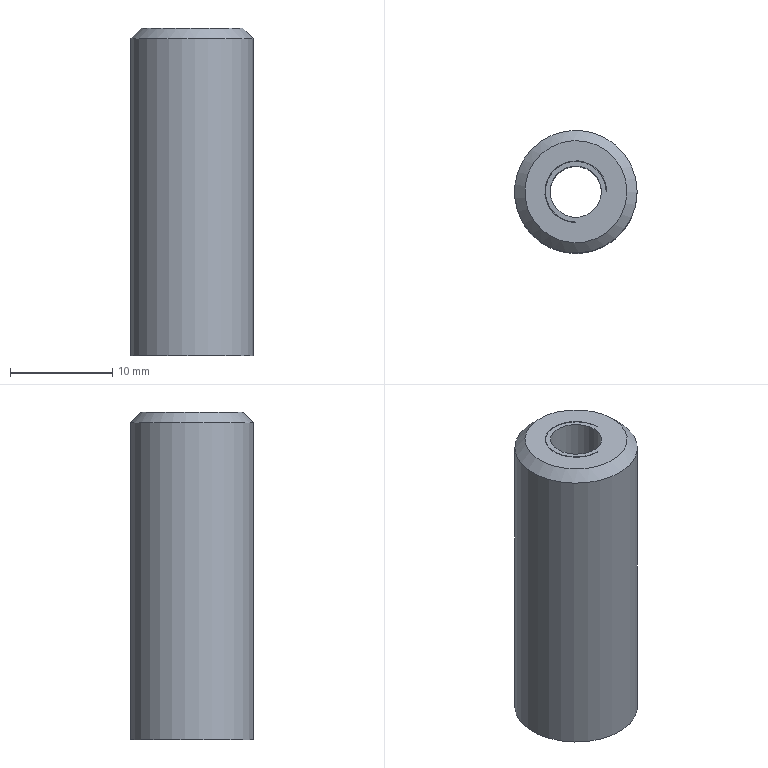Part | STEP file | Tube necking machine_id26_x_t | 1 solid | 9 faces | box 12 x 12 x 32 mm | volume 2950 mm3 | cylinder 4 | plane 4 | cone 1 | commonest cylinder face diameters 5 x1 5.95 x1 6.05 x1 12 x1
STEP:
#1=CARTESIAN_POINT('',(0.,0.,0.));
#2=DIRECTION('',(0.,0.,1.));
#3=DIRECTION('',(1.,0.,0.));
#4=AXIS2_PLACEMENT_3D('',#1,#2,#3);
#5=CARTESIAN_POINT('',(2.975,50.,73.));
#6=VERTEX_POINT('',#5);
#7=CARTESIAN_POINT('',(2.975,50.,105.));
#8=VERTEX_POINT('',#7);
#9=CARTESIAN_POINT('',(2.975,50.,92.));
#10=DIRECTION('',(0.,0.,1.));
#11=VECTOR('',#10,1.);
#12=LINE('',#9,#11);
#13=CARTESIAN_POINT('',(0.,50.,92.));
#14=DIRECTION('',(0.,0.,-1.));
#15=DIRECTION('',(1.,0.,0.));
#16=AXIS2_PLACEMENT_3D('',#13,#14,#15);
#17=CYLINDRICAL_SURFACE('',#16,2.975);
#18=CARTESIAN_POINT('',(6.283,0.));
#19=DIRECTION('',(0.,-1.));
#20=VECTOR('',#19,1.);
#21=LINE('',#18,#20);
#22=(GEOMETRIC_REPRESENTATION_CONTEXT(2)PARAMETRIC_REPRESENTATION_CONTEXT()REPRESENTATION_CONTEXT('',''));
#23=DEFINITIONAL_REPRESENTATION('',(#21),#22);
#24=PCURVE('',#17,#23);
#25=CARTESIAN_POINT('',(3.,50.,85.5));
#26=DIRECTION('',(0.,-1.,0.));
#27=DIRECTION('',(0.,0.,-1.));
#28=AXIS2_PLACEMENT_3D('',#25,#26,#27);
#29=PLANE('',#28);
#30=CARTESIAN_POINT('',(-6.5,-0.025));
#31=DIRECTION('',(-1.,0.));
#32=VECTOR('',#31,1.);
#33=LINE('',#30,#32);
#34=(GEOMETRIC_REPRESENTATION_CONTEXT(2)PARAMETRIC_REPRESENTATION_CONTEXT()REPRESENTATION_CONTEXT('',''));
#35=DEFINITIONAL_REPRESENTATION('',(#33),#34);
#36=PCURVE('',#29,#35);
#37=SURFACE_CURVE('',#12,(#24,#36),.PCURVE_S1.);
#38=EDGE_CURVE('',#6,#8,#37,.T.);
#39=ORIENTED_EDGE('',*,*,#38,.F.);
#40=CARTESIAN_POINT('',(0.,47.025,73.));
#41=VERTEX_POINT('',#40);
#42=CARTESIAN_POINT('',(0.,50.,73.));
#43=DIRECTION('',(0.,0.,1.));
#44=DIRECTION('',(1.,0.,0.));
#45=AXIS2_PLACEMENT_3D('',#42,#43,#44);
#46=CIRCLE('',#45,2.975);
#47=CARTESIAN_POINT('',(6.283,19.));
#48=DIRECTION('',(-1.,0.));
#49=VECTOR('',#48,1.);
#50=LINE('',#47,#49);
#51=(GEOMETRIC_REPRESENTATION_CONTEXT(2)PARAMETRIC_REPRESENTATION_CONTEXT()REPRESENTATION_CONTEXT('',''));
#52=DEFINITIONAL_REPRESENTATION('',(#50),#51);
#53=PCURVE('',#17,#52);
#54=CARTESIAN_POINT('',(0.,50.,73.));
#55=DIRECTION('',(0.,0.,1.));
#56=DIRECTION('',(1.,0.,0.));
#57=AXIS2_PLACEMENT_3D('',#54,#55,#56);
#58=PLANE('',#57);
#59=CARTESIAN_POINT('',(0.,0.));
#60=DIRECTION('',(1.,0.));
#61=AXIS2_PLACEMENT_2D('',#59,#60);
#62=CIRCLE('',#61,2.975);
#63=(GEOMETRIC_REPRESENTATION_CONTEXT(2)PARAMETRIC_REPRESENTATION_CONTEXT()REPRESENTATION_CONTEXT('',''));
#64=DEFINITIONAL_REPRESENTATION('',(#62),#63);
#65=PCURVE('',#58,#64);
#66=SURFACE_CURVE('',#46,(#53,#65),.PCURVE_S1.);
#67=EDGE_CURVE('',#6,#41,#66,.T.);
#68=ORIENTED_EDGE('',*,*,#67,.T.);
#69=CARTESIAN_POINT('',(0.,47.025,105.));
#70=VERTEX_POINT('',#69);
#71=CARTESIAN_POINT('',(0.,47.025,92.));
#72=DIRECTION('',(0.,0.,1.));
#73=VECTOR('',#72,1.);
#74=LINE('',#71,#73);
#75=CARTESIAN_POINT('',(1.571,0.));
#76=DIRECTION('',(0.,-1.));
#77=VECTOR('',#76,1.);
#78=LINE('',#75,#77);
#79=(GEOMETRIC_REPRESENTATION_CONTEXT(2)PARAMETRIC_REPRESENTATION_CONTEXT()REPRESENTATION_CONTEXT('',''));
#80=DEFINITIONAL_REPRESENTATION('',(#78),#79);
#81=PCURVE('',#17,#80);
#82=CARTESIAN_POINT('',(0.,47.,85.5));
#83=DIRECTION('',(-1.,0.,0.));
#84=DIRECTION('',(0.,0.,-1.));
#85=AXIS2_PLACEMENT_3D('',#82,#83,#84);
#86=PLANE('',#85);
#87=CARTESIAN_POINT('',(-6.5,-0.025));
#88=DIRECTION('',(-1.,0.));
#89=VECTOR('',#88,1.);
#90=LINE('',#87,#89);
#91=(GEOMETRIC_REPRESENTATION_CONTEXT(2)PARAMETRIC_REPRESENTATION_CONTEXT()REPRESENTATION_CONTEXT('',''));
#92=DEFINITIONAL_REPRESENTATION('',(#90),#91);
#93=PCURVE('',#86,#92);
#94=SURFACE_CURVE('',#74,(#81,#93),.PCURVE_S1.);
#95=EDGE_CURVE('',#41,#70,#94,.T.);
#96=ORIENTED_EDGE('',*,*,#95,.T.);
#97=CARTESIAN_POINT('',(0.,50.,105.));
#98=DIRECTION('',(0.,0.,1.));
#99=DIRECTION('',(1.,0.,0.));
#100=AXIS2_PLACEMENT_3D('',#97,#98,#99);
#101=CIRCLE('',#100,2.975);
#102=CARTESIAN_POINT('',(6.283,-13.));
#103=DIRECTION('',(-1.,0.));
#104=VECTOR('',#103,1.);
#105=LINE('',#102,#104);
#106=(GEOMETRIC_REPRESENTATION_CONTEXT(2)PARAMETRIC_REPRESENTATION_CONTEXT()REPRESENTATION_CONTEXT('',''));
#107=DEFINITIONAL_REPRESENTATION('',(#105),#106);
#108=PCURVE('',#17,#107);
#109=CARTESIAN_POINT('',(0.,50.,105.));
#110=DIRECTION('',(0.,0.,1.));
#111=DIRECTION('',(1.,0.,0.));
#112=AXIS2_PLACEMENT_3D('',#109,#110,#111);
#113=PLANE('',#112);
#114=CARTESIAN_POINT('',(0.,0.));
#115=DIRECTION('',(1.,0.));
#116=AXIS2_PLACEMENT_2D('',#114,#115);
#117=CIRCLE('',#116,2.975);
#118=(GEOMETRIC_REPRESENTATION_CONTEXT(2)PARAMETRIC_REPRESENTATION_CONTEXT()REPRESENTATION_CONTEXT('',''));
#119=DEFINITIONAL_REPRESENTATION('',(#117),#118);
#120=PCURVE('',#113,#119);
#121=SURFACE_CURVE('',#101,(#108,#120),.PCURVE_S1.);
#122=EDGE_CURVE('',#8,#70,#121,.T.);
#123=ORIENTED_EDGE('',*,*,#122,.F.);
#124=EDGE_LOOP('',(#39,#68,#96,#123));
#125=FACE_BOUND('',#124,.T.);
#126=ADVANCED_FACE('',(#125),#17,.T.);
#127=CARTESIAN_POINT('',(0.,46.975,73.));
#128=VERTEX_POINT('',#127);
#129=CARTESIAN_POINT('',(0.,46.975,105.));
#130=VERTEX_POINT('',#129);
#131=CARTESIAN_POINT('',(0.,46.975,92.));
#132=DIRECTION('',(0.,0.,1.));
#133=VECTOR('',#132,1.);
#134=LINE('',#131,#133);
#135=CARTESIAN_POINT('',(0.,50.,92.));
#136=DIRECTION('',(0.,0.,-1.));
#137=DIRECTION('',(1.,0.,0.));
#138=AXIS2_PLACEMENT_3D('',#135,#136,#137);
#139=CYLINDRICAL_SURFACE('',#138,3.025);
#140=CARTESIAN_POINT('',(1.571,0.));
#141=DIRECTION('',(0.,-1.));
#142=VECTOR('',#141,1.);
#143=LINE('',#140,#142);
#144=(GEOMETRIC_REPRESENTATION_CONTEXT(2)PARAMETRIC_REPRESENTATION_CONTEXT()REPRESENTATION_CONTEXT('',''));
#145=DEFINITIONAL_REPRESENTATION('',(#143),#144);
#146=PCURVE('',#139,#145);
#147=CARTESIAN_POINT('',(-6.5,0.025));
#148=DIRECTION('',(-1.,0.));
#149=VECTOR('',#148,1.);
#150=LINE('',#147,#149);
#151=(GEOMETRIC_REPRESENTATION_CONTEXT(2)PARAMETRIC_REPRESENTATION_CONTEXT()REPRESENTATION_CONTEXT('',''));
#152=DEFINITIONAL_REPRESENTATION('',(#150),#151);
#153=PCURVE('',#86,#152);
#154=SURFACE_CURVE('',#134,(#146,#153),.PCURVE_S1.);
#155=EDGE_CURVE('',#128,#130,#154,.T.);
#156=ORIENTED_EDGE('',*,*,#155,.T.);
#157=CARTESIAN_POINT('',(3.025,50.,105.));
#158=VERTEX_POINT('',#157);
#159=CARTESIAN_POINT('',(0.,50.,105.));
#160=DIRECTION('',(0.,0.,1.));
#161=DIRECTION('',(1.,0.,0.));
#162=AXIS2_PLACEMENT_3D('',#159,#160,#161);
#163=CIRCLE('',#162,3.025);
#164=CARTESIAN_POINT('',(6.283,-13.));
#165=DIRECTION('',(-1.,0.));
#166=VECTOR('',#165,1.);
#167=LINE('',#164,#166);
#168=(GEOMETRIC_REPRESENTATION_CONTEXT(2)PARAMETRIC_REPRESENTATION_CONTEXT()REPRESENTATION_CONTEXT('',''));
#169=DEFINITIONAL_REPRESENTATION('',(#167),#168);
#170=PCURVE('',#139,#169);
#171=CARTESIAN_POINT('',(0.,0.));
#172=DIRECTION('',(1.,0.));
#173=AXIS2_PLACEMENT_2D('',#171,#172);
#174=CIRCLE('',#173,3.025);
#175=(GEOMETRIC_REPRESENTATION_CONTEXT(2)PARAMETRIC_REPRESENTATION_CONTEXT()REPRESENTATION_CONTEXT('',''));
#176=DEFINITIONAL_REPRESENTATION('',(#174),#175);
#177=PCURVE('',#113,#176);
#178=SURFACE_CURVE('',#163,(#170,#177),.PCURVE_S1.);
#179=EDGE_CURVE('',#158,#130,#178,.T.);
#180=ORIENTED_EDGE('',*,*,#179,.F.);
#181=CARTESIAN_POINT('',(3.025,50.,73.));
#182=VERTEX_POINT('',#181);
#183=CARTESIAN_POINT('',(3.025,50.,92.));
#184=DIRECTION('',(0.,0.,1.));
#185=VECTOR('',#184,1.);
#186=LINE('',#183,#185);
#187=CARTESIAN_POINT('',(6.283,0.));
#188=DIRECTION('',(0.,-1.));
#189=VECTOR('',#188,1.);
#190=LINE('',#187,#189);
#191=(GEOMETRIC_REPRESENTATION_CONTEXT(2)PARAMETRIC_REPRESENTATION_CONTEXT()REPRESENTATION_CONTEXT('',''));
#192=DEFINITIONAL_REPRESENTATION('',(#190),#191);
#193=PCURVE('',#139,#192);
#194=CARTESIAN_POINT('',(-6.5,0.025));
#195=DIRECTION('',(-1.,0.));
#196=VECTOR('',#195,1.);
#197=LINE('',#194,#196);
#198=(GEOMETRIC_REPRESENTATION_CONTEXT(2)PARAMETRIC_REPRESENTATION_CONTEXT()REPRESENTATION_CONTEXT('',''));
#199=DEFINITIONAL_REPRESENTATION('',(#197),#198);
#200=PCURVE('',#29,#199);
#201=SURFACE_CURVE('',#186,(#193,#200),.PCURVE_S1.);
#202=EDGE_CURVE('',#182,#158,#201,.T.);
#203=ORIENTED_EDGE('',*,*,#202,.F.);
#204=CARTESIAN_POINT('',(0.,50.,73.));
#205=DIRECTION('',(0.,0.,1.));
#206=DIRECTION('',(1.,0.,0.));
#207=AXIS2_PLACEMENT_3D('',#204,#205,#206);
#208=CIRCLE('',#207,3.025);
#209=CARTESIAN_POINT('',(6.283,19.));
#210=DIRECTION('',(-1.,0.));
#211=VECTOR('',#210,1.);
#212=LINE('',#209,#211);
#213=(GEOMETRIC_REPRESENTATION_CONTEXT(2)PARAMETRIC_REPRESENTATION_CONTEXT()REPRESENTATION_CONTEXT('',''));
#214=DEFINITIONAL_REPRESENTATION('',(#212),#213);
#215=PCURVE('',#139,#214);
#216=CARTESIAN_POINT('',(0.,0.));
#217=DIRECTION('',(1.,0.));
#218=AXIS2_PLACEMENT_2D('',#216,#217);
#219=CIRCLE('',#218,3.025);
#220=(GEOMETRIC_REPRESENTATION_CONTEXT(2)PARAMETRIC_REPRESENTATION_CONTEXT()REPRESENTATION_CONTEXT('',''));
#221=DEFINITIONAL_REPRESENTATION('',(#219),#220);
#222=PCURVE('',#58,#221);
#223=SURFACE_CURVE('',#208,(#215,#222),.PCURVE_S1.);
#224=EDGE_CURVE('',#182,#128,#223,.T.);
#225=ORIENTED_EDGE('',*,*,#224,.T.);
#226=EDGE_LOOP('',(#156,#180,#203,#225));
#227=FACE_BOUND('',#226,.F.);
#228=ADVANCED_FACE('',(#227),#139,.F.);
#229=ORIENTED_EDGE('',*,*,#202,.F.);
#230=CARTESIAN_POINT('',(3.,50.,73.));
#231=DIRECTION('',(-1.,0.,0.));
#232=VECTOR('',#231,1.);
#233=LINE('',#230,#232);
#234=CARTESIAN_POINT('',(12.5,0.));
#235=DIRECTION('',(0.,-1.));
#236=VECTOR('',#235,1.);
#237=LINE('',#234,#236);
#238=(GEOMETRIC_REPRESENTATION_CONTEXT(2)PARAMETRIC_REPRESENTATION_CONTEXT()REPRESENTATION_CONTEXT('',''));
#239=DEFINITIONAL_REPRESENTATION('',(#237),#238);
#240=PCURVE('',#29,#239);
#241=CARTESIAN_POINT('',(3.,0.));
#242=DIRECTION('',(-1.,0.));
#243=VECTOR('',#242,1.);
#244=LINE('',#241,#243);
#245=(GEOMETRIC_REPRESENTATION_CONTEXT(2)PARAMETRIC_REPRESENTATION_CONTEXT()REPRESENTATION_CONTEXT('',''));
#246=DEFINITIONAL_REPRESENTATION('',(#244),#245);
#247=PCURVE('',#58,#246);
#248=SURFACE_CURVE('',#233,(#240,#247),.PCURVE_S1.);
#249=EDGE_CURVE('',#182,#6,#248,.T.);
#250=ORIENTED_EDGE('',*,*,#249,.T.);
#251=ORIENTED_EDGE('',*,*,#38,.T.);
#252=CARTESIAN_POINT('',(3.,50.,105.));
#253=DIRECTION('',(-1.,0.,0.));
#254=VECTOR('',#253,1.);
#255=LINE('',#252,#254);
#256=CARTESIAN_POINT('',(-19.5,0.));
#257=DIRECTION('',(0.,-1.));
#258=VECTOR('',#257,1.);
#259=LINE('',#256,#258);
#260=(GEOMETRIC_REPRESENTATION_CONTEXT(2)PARAMETRIC_REPRESENTATION_CONTEXT()REPRESENTATION_CONTEXT('',''));
#261=DEFINITIONAL_REPRESENTATION('',(#259),#260);
#262=PCURVE('',#29,#261);
#263=CARTESIAN_POINT('',(3.,0.));
#264=DIRECTION('',(-1.,0.));
#265=VECTOR('',#264,1.);
#266=LINE('',#263,#265);
#267=(GEOMETRIC_REPRESENTATION_CONTEXT(2)PARAMETRIC_REPRESENTATION_CONTEXT()REPRESENTATION_CONTEXT('',''));
#268=DEFINITIONAL_REPRESENTATION('',(#266),#267);
#269=PCURVE('',#113,#268);
#270=SURFACE_CURVE('',#255,(#262,#269),.PCURVE_S1.);
#271=EDGE_CURVE('',#158,#8,#270,.T.);
#272=ORIENTED_EDGE('',*,*,#271,.F.);
#273=EDGE_LOOP('',(#229,#250,#251,#272));
#274=FACE_BOUND('',#273,.T.);
#275=ADVANCED_FACE('',(#274),#29,.F.);
#276=ORIENTED_EDGE('',*,*,#95,.F.);
#277=CARTESIAN_POINT('',(0.,47.,73.));
#278=DIRECTION('',(0.,-1.,0.));
#279=VECTOR('',#278,1.);
#280=LINE('',#277,#279);
#281=CARTESIAN_POINT('',(12.5,0.));
#282=DIRECTION('',(0.,1.));
#283=VECTOR('',#282,1.);
#284=LINE('',#281,#283);
#285=(GEOMETRIC_REPRESENTATION_CONTEXT(2)PARAMETRIC_REPRESENTATION_CONTEXT()REPRESENTATION_CONTEXT('',''));
#286=DEFINITIONAL_REPRESENTATION('',(#284),#285);
#287=PCURVE('',#86,#286);
#288=CARTESIAN_POINT('',(0.,-3.));
#289=DIRECTION('',(0.,-1.));
#290=VECTOR('',#289,1.);
#291=LINE('',#288,#290);
#292=(GEOMETRIC_REPRESENTATION_CONTEXT(2)PARAMETRIC_REPRESENTATION_CONTEXT()REPRESENTATION_CONTEXT('',''));
#293=DEFINITIONAL_REPRESENTATION('',(#291),#292);
#294=PCURVE('',#58,#293);
#295=SURFACE_CURVE('',#280,(#287,#294),.PCURVE_S1.);
#296=EDGE_CURVE('',#41,#128,#295,.T.);
#297=ORIENTED_EDGE('',*,*,#296,.T.);
#298=ORIENTED_EDGE('',*,*,#155,.T.);
#299=CARTESIAN_POINT('',(0.,47.,105.));
#300=DIRECTION('',(0.,-1.,0.));
#301=VECTOR('',#300,1.);
#302=LINE('',#299,#301);
#303=CARTESIAN_POINT('',(-19.5,0.));
#304=DIRECTION('',(0.,1.));
#305=VECTOR('',#304,1.);
#306=LINE('',#303,#305);
#307=(GEOMETRIC_REPRESENTATION_CONTEXT(2)PARAMETRIC_REPRESENTATION_CONTEXT()REPRESENTATION_CONTEXT('',''));
#308=DEFINITIONAL_REPRESENTATION('',(#306),#307);
#309=PCURVE('',#86,#308);
#310=CARTESIAN_POINT('',(0.,-3.));
#311=DIRECTION('',(0.,-1.));
#312=VECTOR('',#311,1.);
#313=LINE('',#310,#312);
#314=(GEOMETRIC_REPRESENTATION_CONTEXT(2)PARAMETRIC_REPRESENTATION_CONTEXT()REPRESENTATION_CONTEXT('',''));
#315=DEFINITIONAL_REPRESENTATION('',(#313),#314);
#316=PCURVE('',#113,#315);
#317=SURFACE_CURVE('',#302,(#309,#316),.PCURVE_S1.);
#318=EDGE_CURVE('',#70,#130,#317,.T.);
#319=ORIENTED_EDGE('',*,*,#318,.F.);
#320=EDGE_LOOP('',(#276,#297,#298,#319));
#321=FACE_BOUND('',#320,.T.);
#322=ADVANCED_FACE('',(#321),#86,.T.);
#323=CARTESIAN_POINT('',(5.,50.,105.));
#324=VERTEX_POINT('',#323);
#325=CARTESIAN_POINT('',(0.,50.,105.));
#326=DIRECTION('',(0.,0.,1.));
#327=DIRECTION('',(1.,0.,0.));
#328=AXIS2_PLACEMENT_3D('',#325,#326,#327);
#329=CIRCLE('',#328,5.);
#330=CARTESIAN_POINT('',(0.,0.));
#331=DIRECTION('',(1.,0.));
#332=AXIS2_PLACEMENT_2D('',#330,#331);
#333=CIRCLE('',#332,5.);
#334=(GEOMETRIC_REPRESENTATION_CONTEXT(2)PARAMETRIC_REPRESENTATION_CONTEXT()REPRESENTATION_CONTEXT('',''));
#335=DEFINITIONAL_REPRESENTATION('',(#333),#334);
#336=PCURVE('',#113,#335);
#337=CARTESIAN_POINT('',(0.,50.,104.));
#338=DIRECTION('',(0.,0.,-1.));
#339=DIRECTION('',(-1.,0.,0.));
#340=AXIS2_PLACEMENT_3D('',#337,#338,#339);
#341=CONICAL_SURFACE('',#340,6.,0.7854);
#342=CARTESIAN_POINT('',(9.425,-1.));
#343=DIRECTION('',(-1.,0.));
#344=VECTOR('',#343,1.);
#345=LINE('',#342,#344);
#346=(GEOMETRIC_REPRESENTATION_CONTEXT(2)PARAMETRIC_REPRESENTATION_CONTEXT()REPRESENTATION_CONTEXT('',''));
#347=DEFINITIONAL_REPRESENTATION('',(#345),#346);
#348=PCURVE('',#341,#347);
#349=SURFACE_CURVE('',#329,(#336,#348),.PCURVE_S1.);
#350=EDGE_CURVE('',#324,#324,#349,.T.);
#351=ORIENTED_EDGE('',*,*,#350,.T.);
#352=EDGE_LOOP('',(#351));
#353=FACE_BOUND('',#352,.T.);
#354=CARTESIAN_POINT('',(2.5,50.,105.));
#355=VERTEX_POINT('',#354);
#356=CARTESIAN_POINT('',(0.,50.,105.));
#357=DIRECTION('',(0.,0.,1.));
#358=DIRECTION('',(1.,0.,0.));
#359=AXIS2_PLACEMENT_3D('',#356,#357,#358);
#360=CIRCLE('',#359,2.5);
#361=CARTESIAN_POINT('',(0.,0.));
#362=DIRECTION('',(1.,0.));
#363=AXIS2_PLACEMENT_2D('',#361,#362);
#364=CIRCLE('',#363,2.5);
#365=(GEOMETRIC_REPRESENTATION_CONTEXT(2)PARAMETRIC_REPRESENTATION_CONTEXT()REPRESENTATION_CONTEXT('',''));
#366=DEFINITIONAL_REPRESENTATION('',(#364),#365);
#367=PCURVE('',#113,#366);
#368=CARTESIAN_POINT('',(0.,50.,80.));
#369=DIRECTION('',(0.,0.,1.));
#370=DIRECTION('',(-1.,0.,0.));
#371=AXIS2_PLACEMENT_3D('',#368,#369,#370);
#372=CYLINDRICAL_SURFACE('',#371,2.5);
#373=CARTESIAN_POINT('',(3.142,25.));
#374=DIRECTION('',(1.,0.));
#375=VECTOR('',#374,1.);
#376=LINE('',#373,#375);
#377=(GEOMETRIC_REPRESENTATION_CONTEXT(2)PARAMETRIC_REPRESENTATION_CONTEXT()REPRESENTATION_CONTEXT('',''));
#378=DEFINITIONAL_REPRESENTATION('',(#376),#377);
#379=PCURVE('',#372,#378);
#380=SURFACE_CURVE('',#360,(#367,#379),.PCURVE_S1.);
#381=EDGE_CURVE('',#355,#355,#380,.T.);
#382=ORIENTED_EDGE('',*,*,#381,.F.);
#383=EDGE_LOOP('',(#382));
#384=FACE_BOUND('',#383,.T.);
#385=ORIENTED_EDGE('',*,*,#179,.F.);
#386=ORIENTED_EDGE('',*,*,#271,.T.);
#387=ORIENTED_EDGE('',*,*,#122,.T.);
#388=ORIENTED_EDGE('',*,*,#318,.T.);
#389=EDGE_LOOP('',(#385,#386,#387,#388));
#390=FACE_BOUND('',#389,.T.);
#391=ADVANCED_FACE('',(#353,#384,#390),#113,.T.);
#392=CARTESIAN_POINT('',(2.5,50.,73.));
#393=VERTEX_POINT('',#392);
#394=CARTESIAN_POINT('',(0.,50.,73.));
#395=DIRECTION('',(0.,0.,1.));
#396=DIRECTION('',(1.,0.,0.));
#397=AXIS2_PLACEMENT_3D('',#394,#395,#396);
#398=CIRCLE('',#397,2.5);
#399=CARTESIAN_POINT('',(3.142,-7.));
#400=DIRECTION('',(1.,0.));
#401=VECTOR('',#400,1.);
#402=LINE('',#399,#401);
#403=(GEOMETRIC_REPRESENTATION_CONTEXT(2)PARAMETRIC_REPRESENTATION_CONTEXT()REPRESENTATION_CONTEXT('',''));
#404=DEFINITIONAL_REPRESENTATION('',(#402),#403);
#405=PCURVE('',#372,#404);
#406=CARTESIAN_POINT('',(0.,0.));
#407=DIRECTION('',(1.,0.));
#408=AXIS2_PLACEMENT_2D('',#406,#407);
#409=CIRCLE('',#408,2.5);
#410=(GEOMETRIC_REPRESENTATION_CONTEXT(2)PARAMETRIC_REPRESENTATION_CONTEXT()REPRESENTATION_CONTEXT('',''));
#411=DEFINITIONAL_REPRESENTATION('',(#409),#410);
#412=PCURVE('',#58,#411);
#413=SURFACE_CURVE('',#398,(#405,#412),.PCURVE_S1.);
#414=EDGE_CURVE('',#393,#393,#413,.T.);
#415=ORIENTED_EDGE('',*,*,#414,.T.);
#416=CARTESIAN_POINT('',(2.5,50.,73.));
#417=CARTESIAN_POINT('',(2.5,50.,105.));
#418=B_SPLINE_CURVE_WITH_KNOTS('',1,(#416,#417),.UNSPECIFIED.,.F.,.F.,(2,2),(-7.,25.),.PIECEWISE_BEZIER_KNOTS.);
#419=CARTESIAN_POINT('',(9.425,0.));
#420=DIRECTION('',(0.,1.));
#421=VECTOR('',#420,1.);
#422=LINE('',#419,#421);
#423=(GEOMETRIC_REPRESENTATION_CONTEXT(2)PARAMETRIC_REPRESENTATION_CONTEXT()REPRESENTATION_CONTEXT('',''));
#424=DEFINITIONAL_REPRESENTATION('',(#422),#423);
#425=PCURVE('',#372,#424);
#426=CARTESIAN_POINT('',(3.142,0.));
#427=DIRECTION('',(0.,1.));
#428=VECTOR('',#427,1.);
#429=LINE('',#426,#428);
#430=(GEOMETRIC_REPRESENTATION_CONTEXT(2)PARAMETRIC_REPRESENTATION_CONTEXT()REPRESENTATION_CONTEXT('',''));
#431=DEFINITIONAL_REPRESENTATION('',(#429),#430);
#432=PCURVE('',#372,#431);
#433=SEAM_CURVE('',#418,(#425,#432),.PCURVE_S1.);
#434=EDGE_CURVE('',#393,#355,#433,.T.);
#435=ORIENTED_EDGE('',*,*,#434,.T.);
#436=ORIENTED_EDGE('',*,*,#381,.F.);
#437=ORIENTED_EDGE('',*,*,#434,.F.);
#438=EDGE_LOOP('',(#415,#435,#436,#437));
#439=FACE_BOUND('',#438,.F.);
#440=ADVANCED_FACE('',(#439),#372,.F.);
#441=ORIENTED_EDGE('',*,*,#350,.F.);
#442=CARTESIAN_POINT('',(6.,50.,104.));
#443=VERTEX_POINT('',#442);
#444=CARTESIAN_POINT('',(5.,50.,105.));
#445=CARTESIAN_POINT('',(6.,50.,104.));
#446=B_SPLINE_CURVE_WITH_KNOTS('',1,(#444,#445),.UNSPECIFIED.,.F.,.F.,(2,2),(-1.414,0.),.PIECEWISE_BEZIER_KNOTS.);
#447=CARTESIAN_POINT('',(9.425,0.));
#448=DIRECTION('',(0.,1.));
#449=VECTOR('',#448,1.);
#450=LINE('',#447,#449);
#451=(GEOMETRIC_REPRESENTATION_CONTEXT(2)PARAMETRIC_REPRESENTATION_CONTEXT()REPRESENTATION_CONTEXT('',''));
#452=DEFINITIONAL_REPRESENTATION('',(#450),#451);
#453=PCURVE('',#341,#452);
#454=CARTESIAN_POINT('',(3.142,0.));
#455=DIRECTION('',(0.,1.));
#456=VECTOR('',#455,1.);
#457=LINE('',#454,#456);
#458=(GEOMETRIC_REPRESENTATION_CONTEXT(2)PARAMETRIC_REPRESENTATION_CONTEXT()REPRESENTATION_CONTEXT('',''));
#459=DEFINITIONAL_REPRESENTATION('',(#457),#458);
#460=PCURVE('',#341,#459);
#461=SEAM_CURVE('',#446,(#453,#460),.PCURVE_S1.);
#462=EDGE_CURVE('',#324,#443,#461,.T.);
#463=ORIENTED_EDGE('',*,*,#462,.T.);
#464=CARTESIAN_POINT('',(0.,50.,104.));
#465=DIRECTION('',(0.,0.,-1.));
#466=DIRECTION('',(1.,0.,0.));
#467=AXIS2_PLACEMENT_3D('',#464,#465,#466);
#468=CIRCLE('',#467,6.);
#469=CARTESIAN_POINT('',(3.142,0.));
#470=DIRECTION('',(1.,0.));
#471=VECTOR('',#470,1.);
#472=LINE('',#469,#471);
#473=(GEOMETRIC_REPRESENTATION_CONTEXT(2)PARAMETRIC_REPRESENTATION_CONTEXT()REPRESENTATION_CONTEXT('',''));
#474=DEFINITIONAL_REPRESENTATION('',(#472),#473);
#475=PCURVE('',#341,#474);
#476=CARTESIAN_POINT('',(0.,50.,80.));
#477=DIRECTION('',(0.,0.,1.));
#478=DIRECTION('',(-1.,0.,0.));
#479=AXIS2_PLACEMENT_3D('',#476,#477,#478);
#480=CYLINDRICAL_SURFACE('',#479,6.);
#481=CARTESIAN_POINT('',(9.425,24.));
#482=DIRECTION('',(-1.,0.));
#483=VECTOR('',#482,1.);
#484=LINE('',#481,#483);
#485=(GEOMETRIC_REPRESENTATION_CONTEXT(2)PARAMETRIC_REPRESENTATION_CONTEXT()REPRESENTATION_CONTEXT('',''));
#486=DEFINITIONAL_REPRESENTATION('',(#484),#485);
#487=PCURVE('',#480,#486);
#488=SURFACE_CURVE('',#468,(#475,#487),.PCURVE_S1.);
#489=EDGE_CURVE('',#443,#443,#488,.T.);
#490=ORIENTED_EDGE('',*,*,#489,.F.);
#491=ORIENTED_EDGE('',*,*,#462,.F.);
#492=EDGE_LOOP('',(#441,#463,#490,#491));
#493=FACE_BOUND('',#492,.T.);
#494=ADVANCED_FACE('',(#493),#341,.T.);
#495=ORIENTED_EDGE('',*,*,#489,.T.);
#496=CARTESIAN_POINT('',(6.,50.,73.));
#497=VERTEX_POINT('',#496);
#498=CARTESIAN_POINT('',(6.,50.,73.));
#499=CARTESIAN_POINT('',(6.,50.,104.));
#500=B_SPLINE_CURVE_WITH_KNOTS('',1,(#498,#499),.UNSPECIFIED.,.F.,.F.,(2,2),(-7.,24.),.PIECEWISE_BEZIER_KNOTS.);
#501=CARTESIAN_POINT('',(3.142,0.));
#502=DIRECTION('',(0.,1.));
#503=VECTOR('',#502,1.);
#504=LINE('',#501,#503);
#505=(GEOMETRIC_REPRESENTATION_CONTEXT(2)PARAMETRIC_REPRESENTATION_CONTEXT()REPRESENTATION_CONTEXT('',''));
#506=DEFINITIONAL_REPRESENTATION('',(#504),#505);
#507=PCURVE('',#480,#506);
#508=CARTESIAN_POINT('',(9.425,0.));
#509=DIRECTION('',(0.,1.));
#510=VECTOR('',#509,1.);
#511=LINE('',#508,#510);
#512=(GEOMETRIC_REPRESENTATION_CONTEXT(2)PARAMETRIC_REPRESENTATION_CONTEXT()REPRESENTATION_CONTEXT('',''));
#513=DEFINITIONAL_REPRESENTATION('',(#511),#512);
#514=PCURVE('',#480,#513);
#515=SEAM_CURVE('',#500,(#507,#514),.PCURVE_S1.);
#516=EDGE_CURVE('',#497,#443,#515,.T.);
#517=ORIENTED_EDGE('',*,*,#516,.F.);
#518=CARTESIAN_POINT('',(0.,50.,73.));
#519=DIRECTION('',(0.,0.,1.));
#520=DIRECTION('',(1.,0.,0.));
#521=AXIS2_PLACEMENT_3D('',#518,#519,#520);
#522=CIRCLE('',#521,6.);
#523=CARTESIAN_POINT('',(3.142,-7.));
#524=DIRECTION('',(1.,0.));
#525=VECTOR('',#524,1.);
#526=LINE('',#523,#525);
#527=(GEOMETRIC_REPRESENTATION_CONTEXT(2)PARAMETRIC_REPRESENTATION_CONTEXT()REPRESENTATION_CONTEXT('',''));
#528=DEFINITIONAL_REPRESENTATION('',(#526),#527);
#529=PCURVE('',#480,#528);
#530=CARTESIAN_POINT('',(0.,0.));
#531=DIRECTION('',(1.,0.));
#532=AXIS2_PLACEMENT_2D('',#530,#531);
#533=CIRCLE('',#532,6.);
#534=(GEOMETRIC_REPRESENTATION_CONTEXT(2)PARAMETRIC_REPRESENTATION_CONTEXT()REPRESENTATION_CONTEXT('',''));
#535=DEFINITIONAL_REPRESENTATION('',(#533),#534);
#536=PCURVE('',#58,#535);
#537=SURFACE_CURVE('',#522,(#529,#536),.PCURVE_S1.);
#538=EDGE_CURVE('',#497,#497,#537,.T.);
#539=ORIENTED_EDGE('',*,*,#538,.T.);
#540=ORIENTED_EDGE('',*,*,#516,.T.);
#541=EDGE_LOOP('',(#495,#517,#539,#540));
#542=FACE_BOUND('',#541,.T.);
#543=ADVANCED_FACE('',(#542),#480,.T.);
#544=ORIENTED_EDGE('',*,*,#414,.T.);
#545=EDGE_LOOP('',(#544));
#546=FACE_BOUND('',#545,.T.);
#547=ORIENTED_EDGE('',*,*,#224,.T.);
#548=ORIENTED_EDGE('',*,*,#296,.F.);
#549=ORIENTED_EDGE('',*,*,#67,.F.);
#550=ORIENTED_EDGE('',*,*,#249,.F.);
#551=EDGE_LOOP('',(#547,#548,#549,#550));
#552=FACE_BOUND('',#551,.T.);
#553=ORIENTED_EDGE('',*,*,#538,.F.);
#554=EDGE_LOOP('',(#553));
#555=FACE_BOUND('',#554,.T.);
#556=ADVANCED_FACE('',(#546,#552,#555),#58,.F.);
#557=CLOSED_SHELL('',(#126,#228,#275,#322,#391,#440,#494,#543,#556));
#558=MANIFOLD_SOLID_BREP('',#557);
#559=(LENGTH_UNIT()NAMED_UNIT(*)SI_UNIT(.MILLI.,.METRE.));
#560=UNCERTAINTY_MEASURE_WITH_UNIT(LENGTH_MEASURE(0.000002),#559,'','');
#561=(NAMED_UNIT(*)PLANE_ANGLE_UNIT()SI_UNIT($,.RADIAN.));
#562=(NAMED_UNIT(*)SI_UNIT($,.STERADIAN.)SOLID_ANGLE_UNIT());
#563=(GEOMETRIC_REPRESENTATION_CONTEXT(3)GLOBAL_UNCERTAINTY_ASSIGNED_CONTEXT((#560))GLOBAL_UNIT_ASSIGNED_CONTEXT((#559,#561,#562))REPRESENTATION_CONTEXT('',''));
#564=ADVANCED_BREP_SHAPE_REPRESENTATION('',(#4,#558),#563);